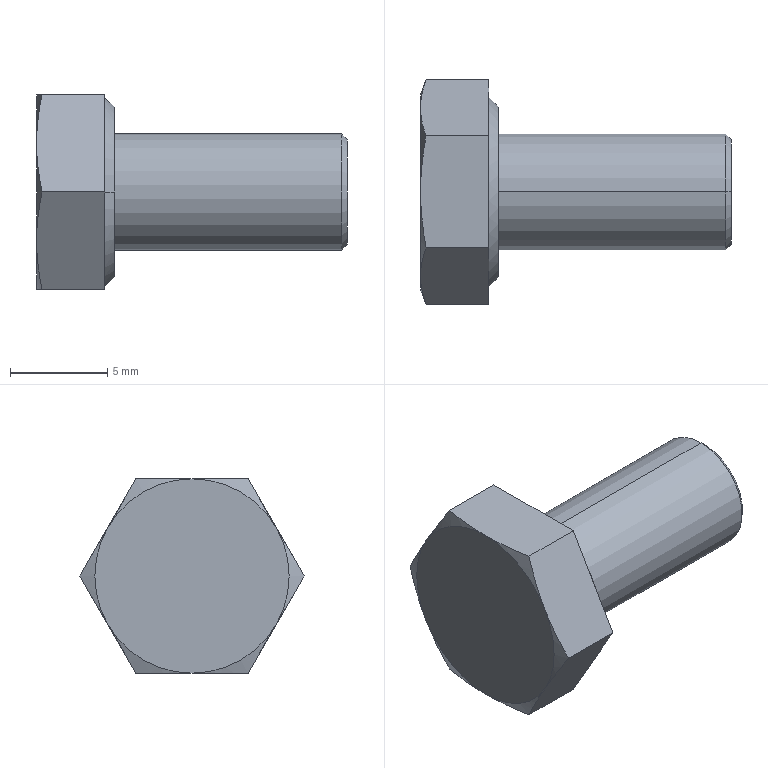Part | STEP file | hex head bolts-full thread grade c gb_GB_FASTENER_BOLT_HHBFTC M6X12-S | 1 solid | 22 faces | box 16 x 11.547 x 10 mm | volume 674.444 mm3 | cone 10 | plane 10 | cylinder 2 | commonest cylinder face diameters 6 x2
STEP:
#1=CARTESIAN_POINT('',(15.7,0.,3.));
#2=VERTEX_POINT('',#1);
#3=CARTESIAN_POINT('',(15.7,0.,-3.));
#4=VERTEX_POINT('',#3);
#5=CARTESIAN_POINT('',(15.7,0.,0.));
#6=DIRECTION('',(-1.,0.,0.));
#7=DIRECTION('',(0.,0.,1.));
#8=AXIS2_PLACEMENT_3D('',#5,#6,#7);
#9=CIRCLE('',#8,3.);
#10=EDGE_CURVE('',#2,#4,#9,.T.);
#11=ORIENTED_EDGE('',*,*,#10,.T.);
#12=CARTESIAN_POINT('',(4.,0.,-3.));
#13=VERTEX_POINT('',#12);
#14=CARTESIAN_POINT('',(16.,0.,-3.));
#15=DIRECTION('',(-1.,0.,0.));
#16=VECTOR('',#15,1000.);
#17=LINE('',#14,#16);
#18=EDGE_CURVE('',#4,#13,#17,.T.);
#19=ORIENTED_EDGE('',*,*,#18,.T.);
#20=CARTESIAN_POINT('',(4.,0.,3.));
#21=VERTEX_POINT('',#20);
#22=CARTESIAN_POINT('',(4.,0.,0.));
#23=DIRECTION('',(1.,0.,0.));
#24=DIRECTION('',(0.,0.,1.));
#25=AXIS2_PLACEMENT_3D('',#22,#23,#24);
#26=CIRCLE('',#25,3.);
#27=EDGE_CURVE('',#13,#21,#26,.T.);
#28=ORIENTED_EDGE('',*,*,#27,.T.);
#29=CARTESIAN_POINT('',(16.,0.,3.));
#30=DIRECTION('',(-1.,0.,0.));
#31=VECTOR('',#30,1000.);
#32=LINE('',#29,#31);
#33=EDGE_CURVE('',#2,#21,#32,.T.);
#34=ORIENTED_EDGE('',*,*,#33,.F.);
#35=EDGE_LOOP('',(#11,#19,#28,#34));
#36=FACE_OUTER_BOUND('',#35,.T.);
#37=CARTESIAN_POINT('',(16.,0.,0.));
#38=DIRECTION('',(-1.,0.,0.));
#39=DIRECTION('',(0.,0.,1.));
#40=AXIS2_PLACEMENT_3D('',#37,#38,#39);
#41=CYLINDRICAL_SURFACE('',#40,3.);
#42=ADVANCED_FACE('',(#36),#41,.T.);
#43=CARTESIAN_POINT('',(16.,0.,2.7));
#44=VERTEX_POINT('',#43);
#45=CARTESIAN_POINT('',(16.,0.,-2.7));
#46=VERTEX_POINT('',#45);
#47=CARTESIAN_POINT('',(16.,0.,0.));
#48=DIRECTION('',(-1.,0.,0.));
#49=DIRECTION('',(0.,0.,1.));
#50=AXIS2_PLACEMENT_3D('',#47,#48,#49);
#51=CIRCLE('',#50,2.7);
#52=EDGE_CURVE('',#44,#46,#51,.T.);
#53=ORIENTED_EDGE('',*,*,#52,.T.);
#54=CARTESIAN_POINT('',(15.7,0.,-3.));
#55=DIRECTION('',(-0.7071,0.,-0.7071));
#56=VECTOR('',#55,1000.);
#57=LINE('',#54,#56);
#58=EDGE_CURVE('',#46,#4,#57,.T.);
#59=ORIENTED_EDGE('',*,*,#58,.T.);
#60=ORIENTED_EDGE('',*,*,#10,.F.);
#61=CARTESIAN_POINT('',(15.7,0.,3.));
#62=DIRECTION('',(-0.7071,0.,0.7071));
#63=VECTOR('',#62,1000.);
#64=LINE('',#61,#63);
#65=EDGE_CURVE('',#44,#2,#64,.T.);
#66=ORIENTED_EDGE('',*,*,#65,.F.);
#67=EDGE_LOOP('',(#53,#59,#60,#66));
#68=FACE_OUTER_BOUND('',#67,.T.);
#69=CARTESIAN_POINT('',(15.7,0.,0.));
#70=DIRECTION('',(-1.,0.,0.));
#71=DIRECTION('',(0.,0.,1.));
#72=AXIS2_PLACEMENT_3D('',#69,#70,#71);
#73=CONICAL_SURFACE('',#72,3.,0.7854);
#74=ADVANCED_FACE('',(#68),#73,.T.);
#75=CARTESIAN_POINT('',(4.,4.37,0.));
#76=VERTEX_POINT('',#75);
#77=CARTESIAN_POINT('',(4.,-4.37,0.));
#78=VERTEX_POINT('',#77);
#79=CARTESIAN_POINT('',(4.,0.,0.));
#80=DIRECTION('',(1.,0.,0.));
#81=DIRECTION('',(0.,-1.,0.));
#82=AXIS2_PLACEMENT_3D('',#79,#80,#81);
#83=CIRCLE('',#82,4.37);
#84=EDGE_CURVE('',#76,#78,#83,.T.);
#85=ORIENTED_EDGE('',*,*,#84,.F.);
#86=CARTESIAN_POINT('',(3.5,4.87,0.));
#87=VERTEX_POINT('',#86);
#88=CARTESIAN_POINT('',(3.5,4.87,0.));
#89=DIRECTION('',(-0.7071,0.7071,0.));
#90=VECTOR('',#89,1000.);
#91=LINE('',#88,#90);
#92=EDGE_CURVE('',#76,#87,#91,.T.);
#93=ORIENTED_EDGE('',*,*,#92,.T.);
#94=CARTESIAN_POINT('',(3.5,-4.87,0.));
#95=VERTEX_POINT('',#94);
#96=CARTESIAN_POINT('',(3.5,0.,0.));
#97=DIRECTION('',(1.,0.,0.));
#98=DIRECTION('',(0.,-1.,0.));
#99=AXIS2_PLACEMENT_3D('',#96,#97,#98);
#100=CIRCLE('',#99,4.87);
#101=EDGE_CURVE('',#87,#95,#100,.T.);
#102=ORIENTED_EDGE('',*,*,#101,.T.);
#103=CARTESIAN_POINT('',(3.5,-4.87,0.));
#104=DIRECTION('',(-0.7071,-0.7071,0.));
#105=VECTOR('',#104,1000.);
#106=LINE('',#103,#105);
#107=EDGE_CURVE('',#78,#95,#106,.T.);
#108=ORIENTED_EDGE('',*,*,#107,.F.);
#109=EDGE_LOOP('',(#85,#93,#102,#108));
#110=FACE_OUTER_BOUND('',#109,.T.);
#111=CARTESIAN_POINT('',(3.5,0.,0.));
#112=DIRECTION('',(-1.,0.,0.));
#113=DIRECTION('',(0.,-1.,0.));
#114=AXIS2_PLACEMENT_3D('',#111,#112,#113);
#115=CONICAL_SURFACE('',#114,4.87,0.7854);
#116=ADVANCED_FACE('',(#110),#115,.T.);
#117=ORIENTED_EDGE('',*,*,#18,.F.);
#118=CARTESIAN_POINT('',(15.7,0.,0.));
#119=DIRECTION('',(-1.,0.,0.));
#120=DIRECTION('',(0.,0.,1.));
#121=AXIS2_PLACEMENT_3D('',#118,#119,#120);
#122=CIRCLE('',#121,3.);
#123=EDGE_CURVE('',#4,#2,#122,.T.);
#124=ORIENTED_EDGE('',*,*,#123,.T.);
#125=ORIENTED_EDGE('',*,*,#33,.T.);
#126=CARTESIAN_POINT('',(4.,0.,0.));
#127=DIRECTION('',(1.,0.,0.));
#128=DIRECTION('',(0.,0.,1.));
#129=AXIS2_PLACEMENT_3D('',#126,#127,#128);
#130=CIRCLE('',#129,3.);
#131=EDGE_CURVE('',#21,#13,#130,.T.);
#132=ORIENTED_EDGE('',*,*,#131,.T.);
#133=EDGE_LOOP('',(#117,#124,#125,#132));
#134=FACE_OUTER_BOUND('',#133,.T.);
#135=CARTESIAN_POINT('',(16.,0.,0.));
#136=DIRECTION('',(-1.,0.,0.));
#137=DIRECTION('',(0.,0.,1.));
#138=AXIS2_PLACEMENT_3D('',#135,#136,#137);
#139=CYLINDRICAL_SURFACE('',#138,3.);
#140=ADVANCED_FACE('',(#134),#139,.T.);
#141=ORIENTED_EDGE('',*,*,#131,.F.);
#142=ORIENTED_EDGE('',*,*,#27,.F.);
#143=EDGE_LOOP('',(#141,#142));
#144=FACE_BOUND('',#143,.T.);
#145=CARTESIAN_POINT('',(4.,0.,0.));
#146=DIRECTION('',(1.,0.,0.));
#147=DIRECTION('',(0.,-1.,0.));
#148=AXIS2_PLACEMENT_3D('',#145,#146,#147);
#149=CIRCLE('',#148,4.37);
#150=EDGE_CURVE('',#78,#76,#149,.T.);
#151=ORIENTED_EDGE('',*,*,#150,.T.);
#152=ORIENTED_EDGE('',*,*,#84,.T.);
#153=EDGE_LOOP('',(#151,#152));
#154=FACE_OUTER_BOUND('',#153,.T.);
#155=CARTESIAN_POINT('',(4.,-8.66,-5.));
#156=DIRECTION('',(1.,0.,0.));
#157=DIRECTION('',(0.,0.,-1.));
#158=AXIS2_PLACEMENT_3D('',#155,#156,#157);
#159=PLANE('',#158);
#160=ADVANCED_FACE('',(#144,#154),#159,.T.);
#161=ORIENTED_EDGE('',*,*,#58,.F.);
#162=CARTESIAN_POINT('',(16.,0.,0.));
#163=DIRECTION('',(-1.,0.,0.));
#164=DIRECTION('',(0.,0.,1.));
#165=AXIS2_PLACEMENT_3D('',#162,#163,#164);
#166=CIRCLE('',#165,2.7);
#167=EDGE_CURVE('',#46,#44,#166,.T.);
#168=ORIENTED_EDGE('',*,*,#167,.T.);
#169=ORIENTED_EDGE('',*,*,#65,.T.);
#170=ORIENTED_EDGE('',*,*,#123,.F.);
#171=EDGE_LOOP('',(#161,#168,#169,#170));
#172=FACE_OUTER_BOUND('',#171,.T.);
#173=CARTESIAN_POINT('',(15.7,0.,0.));
#174=DIRECTION('',(-1.,0.,0.));
#175=DIRECTION('',(0.,0.,1.));
#176=AXIS2_PLACEMENT_3D('',#173,#174,#175);
#177=CONICAL_SURFACE('',#176,3.,0.7854);
#178=ADVANCED_FACE('',(#172),#177,.T.);
#179=ORIENTED_EDGE('',*,*,#92,.F.);
#180=ORIENTED_EDGE('',*,*,#150,.F.);
#181=ORIENTED_EDGE('',*,*,#107,.T.);
#182=CARTESIAN_POINT('',(3.5,0.,0.));
#183=DIRECTION('',(1.,0.,0.));
#184=DIRECTION('',(0.,-1.,0.));
#185=AXIS2_PLACEMENT_3D('',#182,#183,#184);
#186=CIRCLE('',#185,4.87);
#187=EDGE_CURVE('',#95,#87,#186,.T.);
#188=ORIENTED_EDGE('',*,*,#187,.T.);
#189=EDGE_LOOP('',(#179,#180,#181,#188));
#190=FACE_OUTER_BOUND('',#189,.T.);
#191=CARTESIAN_POINT('',(3.5,0.,0.));
#192=DIRECTION('',(-1.,0.,0.));
#193=DIRECTION('',(0.,-1.,0.));
#194=AXIS2_PLACEMENT_3D('',#191,#192,#193);
#195=CONICAL_SURFACE('',#194,4.87,0.7854);
#196=ADVANCED_FACE('',(#190),#195,.T.);
#197=ORIENTED_EDGE('',*,*,#52,.F.);
#198=ORIENTED_EDGE('',*,*,#167,.F.);
#199=EDGE_LOOP('',(#197,#198));
#200=FACE_OUTER_BOUND('',#199,.T.);
#201=CARTESIAN_POINT('',(16.,0.,0.));
#202=DIRECTION('',(1.,0.,0.));
#203=DIRECTION('',(0.,0.,-1.));
#204=AXIS2_PLACEMENT_3D('',#201,#202,#203);
#205=PLANE('',#204);
#206=ADVANCED_FACE('',(#200),#205,.T.);
#207=CARTESIAN_POINT('',(3.5,5.774,0.));
#208=VERTEX_POINT('',#207);
#209=CARTESIAN_POINT('',(3.5,2.887,5.));
#210=VERTEX_POINT('',#209);
#211=CARTESIAN_POINT('',(3.5,5.774,0.));
#212=DIRECTION('',(0.,-0.5,0.866));
#213=VECTOR('',#212,1000.);
#214=LINE('',#211,#213);
#215=EDGE_CURVE('',#208,#210,#214,.T.);
#216=ORIENTED_EDGE('',*,*,#215,.T.);
#217=CARTESIAN_POINT('',(3.5,-2.887,5.));
#218=VERTEX_POINT('',#217);
#219=CARTESIAN_POINT('',(3.5,4.87,5.));
#220=DIRECTION('',(0.,-1.,0.));
#221=VECTOR('',#220,1000.);
#222=LINE('',#219,#221);
#223=EDGE_CURVE('',#210,#218,#222,.T.);
#224=ORIENTED_EDGE('',*,*,#223,.T.);
#225=CARTESIAN_POINT('',(3.5,-5.774,0.));
#226=VERTEX_POINT('',#225);
#227=CARTESIAN_POINT('',(3.5,-2.887,5.));
#228=DIRECTION('',(0.,-0.5,-0.866));
#229=VECTOR('',#228,1000.);
#230=LINE('',#227,#229);
#231=EDGE_CURVE('',#218,#226,#230,.T.);
#232=ORIENTED_EDGE('',*,*,#231,.T.);
#233=CARTESIAN_POINT('',(3.5,-2.887,-5.));
#234=VERTEX_POINT('',#233);
#235=CARTESIAN_POINT('',(3.5,-5.774,0.));
#236=DIRECTION('',(0.,0.5,-0.866));
#237=VECTOR('',#236,1000.);
#238=LINE('',#235,#237);
#239=EDGE_CURVE('',#226,#234,#238,.T.);
#240=ORIENTED_EDGE('',*,*,#239,.T.);
#241=CARTESIAN_POINT('',(3.5,2.887,-5.));
#242=VERTEX_POINT('',#241);
#243=CARTESIAN_POINT('',(3.5,4.87,-5.));
#244=DIRECTION('',(0.,1.,0.));
#245=VECTOR('',#244,1000.);
#246=LINE('',#243,#245);
#247=EDGE_CURVE('',#234,#242,#246,.T.);
#248=ORIENTED_EDGE('',*,*,#247,.T.);
#249=CARTESIAN_POINT('',(3.5,2.887,-5.));
#250=DIRECTION('',(0.,0.5,0.866));
#251=VECTOR('',#250,1000.);
#252=LINE('',#249,#251);
#253=EDGE_CURVE('',#242,#208,#252,.T.);
#254=ORIENTED_EDGE('',*,*,#253,.T.);
#255=EDGE_LOOP('',(#216,#224,#232,#240,#248,#254));
#256=FACE_OUTER_BOUND('',#255,.T.);
#257=ORIENTED_EDGE('',*,*,#187,.F.);
#258=ORIENTED_EDGE('',*,*,#101,.F.);
#259=EDGE_LOOP('',(#257,#258));
#260=FACE_BOUND('',#259,.T.);
#261=CARTESIAN_POINT('',(3.5,4.87,0.));
#262=DIRECTION('',(1.,0.,0.));
#263=DIRECTION('',(0.,0.,-1.));
#264=AXIS2_PLACEMENT_3D('',#261,#262,#263);
#265=PLANE('',#264);
#266=ADVANCED_FACE('',(#256,#260),#265,.T.);
#267=CARTESIAN_POINT('',(0.2815,-2.887,5.));
#268=VERTEX_POINT('',#267);
#269=CARTESIAN_POINT('',(4.,-2.887,5.));
#270=DIRECTION('',(-1.,0.,0.));
#271=VECTOR('',#270,1000.);
#272=LINE('',#269,#271);
#273=EDGE_CURVE('',#218,#268,#272,.T.);
#274=ORIENTED_EDGE('',*,*,#273,.F.);
#275=ORIENTED_EDGE('',*,*,#223,.F.);
#276=CARTESIAN_POINT('',(0.2815,2.887,5.));
#277=VERTEX_POINT('',#276);
#278=CARTESIAN_POINT('',(4.,2.887,5.));
#279=DIRECTION('',(1.,0.,0.));
#280=VECTOR('',#279,1000.);
#281=LINE('',#278,#280);
#282=EDGE_CURVE('',#277,#210,#281,.T.);
#283=ORIENTED_EDGE('',*,*,#282,.F.);
#284=CARTESIAN_POINT('',(0.,0.,5.));
#285=VERTEX_POINT('',#284);
#286=CARTESIAN_POINT('',(0.,0.,5.));
#287=CARTESIAN_POINT('',(0.,0.9714,5.));
#288=CARTESIAN_POINT('',(0.1078,1.932,5.));
#289=CARTESIAN_POINT('',(0.2815,2.887,5.));
#290=B_SPLINE_CURVE_WITH_KNOTS('',3,(#286,#287,#288,#289),.UNSPECIFIED.,.F.,.F.,(4,4),(0.,0.0029),.UNSPECIFIED.);
#291=EDGE_CURVE('',#285,#277,#290,.T.);
#292=ORIENTED_EDGE('',*,*,#291,.F.);
#293=CARTESIAN_POINT('',(0.2815,-2.887,5.));
#294=CARTESIAN_POINT('',(0.1078,-1.932,5.));
#295=CARTESIAN_POINT('',(0.,-0.9714,5.));
#296=CARTESIAN_POINT('',(0.,0.,5.));
#297=B_SPLINE_CURVE_WITH_KNOTS('',3,(#293,#294,#295,#296),.UNSPECIFIED.,.F.,.F.,(4,4),(0.,0.0029),.UNSPECIFIED.);
#298=EDGE_CURVE('',#268,#285,#297,.T.);
#299=ORIENTED_EDGE('',*,*,#298,.F.);
#300=EDGE_LOOP('',(#274,#275,#283,#292,#299));
#301=FACE_OUTER_BOUND('',#300,.T.);
#302=CARTESIAN_POINT('',(4.,2.887,5.));
#303=DIRECTION('',(0.,0.,-1.));
#304=DIRECTION('',(0.,1.,0.));
#305=AXIS2_PLACEMENT_3D('',#302,#303,#304);
#306=PLANE('',#305);
#307=ADVANCED_FACE('',(#301),#306,.F.);
#308=ORIENTED_EDGE('',*,*,#282,.T.);
#309=ORIENTED_EDGE('',*,*,#215,.F.);
#310=CARTESIAN_POINT('',(0.2815,5.774,0.));
#311=VERTEX_POINT('',#310);
#312=CARTESIAN_POINT('',(4.,5.774,0.));
#313=DIRECTION('',(1.,0.,0.));
#314=VECTOR('',#313,1000.);
#315=LINE('',#312,#314);
#316=EDGE_CURVE('',#311,#208,#315,.T.);
#317=ORIENTED_EDGE('',*,*,#316,.F.);
#318=CARTESIAN_POINT('',(0.,4.33,2.5));
#319=VERTEX_POINT('',#318);
#320=CARTESIAN_POINT('',(0.,4.33,2.5));
#321=CARTESIAN_POINT('',(0.,4.816,1.659));
#322=CARTESIAN_POINT('',(0.1078,5.296,0.8266));
#323=CARTESIAN_POINT('',(0.2815,5.774,0.));
#324=B_SPLINE_CURVE_WITH_KNOTS('',3,(#320,#321,#322,#323),.UNSPECIFIED.,.F.,.F.,(4,4),(0.,0.0029),.UNSPECIFIED.);
#325=EDGE_CURVE('',#319,#311,#324,.T.);
#326=ORIENTED_EDGE('',*,*,#325,.F.);
#327=CARTESIAN_POINT('',(0.2815,2.887,5.));
#328=CARTESIAN_POINT('',(0.1078,3.364,4.173));
#329=CARTESIAN_POINT('',(0.,3.844,3.341));
#330=CARTESIAN_POINT('',(0.,4.33,2.5));
#331=B_SPLINE_CURVE_WITH_KNOTS('',3,(#327,#328,#329,#330),.UNSPECIFIED.,.F.,.F.,(4,4),(0.,0.0029),.UNSPECIFIED.);
#332=EDGE_CURVE('',#277,#319,#331,.T.);
#333=ORIENTED_EDGE('',*,*,#332,.F.);
#334=EDGE_LOOP('',(#308,#309,#317,#326,#333));
#335=FACE_OUTER_BOUND('',#334,.T.);
#336=CARTESIAN_POINT('',(4.,5.774,0.));
#337=DIRECTION('',(0.,-0.866,-0.5));
#338=DIRECTION('',(0.,0.5,-0.866));
#339=AXIS2_PLACEMENT_3D('',#336,#337,#338);
#340=PLANE('',#339);
#341=ADVANCED_FACE('',(#335),#340,.F.);
#342=ORIENTED_EDGE('',*,*,#316,.T.);
#343=ORIENTED_EDGE('',*,*,#253,.F.);
#344=CARTESIAN_POINT('',(0.2815,2.887,-5.));
#345=VERTEX_POINT('',#344);
#346=CARTESIAN_POINT('',(4.,2.887,-5.));
#347=DIRECTION('',(1.,0.,0.));
#348=VECTOR('',#347,1000.);
#349=LINE('',#346,#348);
#350=EDGE_CURVE('',#345,#242,#349,.T.);
#351=ORIENTED_EDGE('',*,*,#350,.F.);
#352=CARTESIAN_POINT('',(0.,4.33,-2.5));
#353=VERTEX_POINT('',#352);
#354=CARTESIAN_POINT('',(0.,4.33,-2.5));
#355=CARTESIAN_POINT('',(0.,3.844,-3.341));
#356=CARTESIAN_POINT('',(0.1078,3.364,-4.173));
#357=CARTESIAN_POINT('',(0.2815,2.887,-5.));
#358=B_SPLINE_CURVE_WITH_KNOTS('',3,(#354,#355,#356,#357),.UNSPECIFIED.,.F.,.F.,(4,4),(0.,0.0029),.UNSPECIFIED.);
#359=EDGE_CURVE('',#353,#345,#358,.T.);
#360=ORIENTED_EDGE('',*,*,#359,.F.);
#361=CARTESIAN_POINT('',(0.2815,5.774,0.));
#362=CARTESIAN_POINT('',(0.1078,5.296,-0.8266));
#363=CARTESIAN_POINT('',(0.,4.816,-1.659));
#364=CARTESIAN_POINT('',(0.,4.33,-2.5));
#365=B_SPLINE_CURVE_WITH_KNOTS('',3,(#361,#362,#363,#364),.UNSPECIFIED.,.F.,.F.,(4,4),(0.,0.0029),.UNSPECIFIED.);
#366=EDGE_CURVE('',#311,#353,#365,.T.);
#367=ORIENTED_EDGE('',*,*,#366,.F.);
#368=EDGE_LOOP('',(#342,#343,#351,#360,#367));
#369=FACE_OUTER_BOUND('',#368,.T.);
#370=CARTESIAN_POINT('',(4.,2.887,-5.));
#371=DIRECTION('',(0.,-0.866,0.5));
#372=DIRECTION('',(0.,-0.5,-0.866));
#373=AXIS2_PLACEMENT_3D('',#370,#371,#372);
#374=PLANE('',#373);
#375=ADVANCED_FACE('',(#369),#374,.F.);
#376=ORIENTED_EDGE('',*,*,#350,.T.);
#377=ORIENTED_EDGE('',*,*,#247,.F.);
#378=CARTESIAN_POINT('',(0.2815,-2.887,-5.));
#379=VERTEX_POINT('',#378);
#380=CARTESIAN_POINT('',(4.,-2.887,-5.));
#381=DIRECTION('',(1.,0.,0.));
#382=VECTOR('',#381,1000.);
#383=LINE('',#380,#382);
#384=EDGE_CURVE('',#379,#234,#383,.T.);
#385=ORIENTED_EDGE('',*,*,#384,.F.);
#386=CARTESIAN_POINT('',(0.,0.,-5.));
#387=VERTEX_POINT('',#386);
#388=CARTESIAN_POINT('',(0.,0.,-5.));
#389=CARTESIAN_POINT('',(0.,-0.9714,-5.));
#390=CARTESIAN_POINT('',(0.1078,-1.932,-5.));
#391=CARTESIAN_POINT('',(0.2815,-2.887,-5.));
#392=B_SPLINE_CURVE_WITH_KNOTS('',3,(#388,#389,#390,#391),.UNSPECIFIED.,.F.,.F.,(4,4),(0.,0.0029),.UNSPECIFIED.);
#393=EDGE_CURVE('',#387,#379,#392,.T.);
#394=ORIENTED_EDGE('',*,*,#393,.F.);
#395=CARTESIAN_POINT('',(0.2815,2.887,-5.));
#396=CARTESIAN_POINT('',(0.1078,1.932,-5.));
#397=CARTESIAN_POINT('',(0.,0.9714,-5.));
#398=CARTESIAN_POINT('',(0.,0.,-5.));
#399=B_SPLINE_CURVE_WITH_KNOTS('',3,(#395,#396,#397,#398),.UNSPECIFIED.,.F.,.F.,(4,4),(0.,0.0029),.UNSPECIFIED.);
#400=EDGE_CURVE('',#345,#387,#399,.T.);
#401=ORIENTED_EDGE('',*,*,#400,.F.);
#402=EDGE_LOOP('',(#376,#377,#385,#394,#401));
#403=FACE_OUTER_BOUND('',#402,.T.);
#404=CARTESIAN_POINT('',(4.,-2.887,-5.));
#405=DIRECTION('',(0.,0.,1.));
#406=DIRECTION('',(1.,0.,0.));
#407=AXIS2_PLACEMENT_3D('',#404,#405,#406);
#408=PLANE('',#407);
#409=ADVANCED_FACE('',(#403),#408,.F.);
#410=ORIENTED_EDGE('',*,*,#384,.T.);
#411=ORIENTED_EDGE('',*,*,#239,.F.);
#412=CARTESIAN_POINT('',(0.2815,-5.774,0.));
#413=VERTEX_POINT('',#412);
#414=CARTESIAN_POINT('',(4.,-5.774,0.));
#415=DIRECTION('',(1.,0.,0.));
#416=VECTOR('',#415,1000.);
#417=LINE('',#414,#416);
#418=EDGE_CURVE('',#413,#226,#417,.T.);
#419=ORIENTED_EDGE('',*,*,#418,.F.);
#420=CARTESIAN_POINT('',(0.,-4.33,-2.5));
#421=VERTEX_POINT('',#420);
#422=CARTESIAN_POINT('',(0.,-4.33,-2.5));
#423=CARTESIAN_POINT('',(0.,-4.816,-1.659));
#424=CARTESIAN_POINT('',(0.1078,-5.296,-0.8266));
#425=CARTESIAN_POINT('',(0.2815,-5.774,0.));
#426=B_SPLINE_CURVE_WITH_KNOTS('',3,(#422,#423,#424,#425),.UNSPECIFIED.,.F.,.F.,(4,4),(0.,0.0029),.UNSPECIFIED.);
#427=EDGE_CURVE('',#421,#413,#426,.T.);
#428=ORIENTED_EDGE('',*,*,#427,.F.);
#429=CARTESIAN_POINT('',(0.2815,-2.887,-5.));
#430=CARTESIAN_POINT('',(0.1078,-3.364,-4.173));
#431=CARTESIAN_POINT('',(0.,-3.844,-3.341));
#432=CARTESIAN_POINT('',(0.,-4.33,-2.5));
#433=B_SPLINE_CURVE_WITH_KNOTS('',3,(#429,#430,#431,#432),.UNSPECIFIED.,.F.,.F.,(4,4),(0.,0.0029),.UNSPECIFIED.);
#434=EDGE_CURVE('',#379,#421,#433,.T.);
#435=ORIENTED_EDGE('',*,*,#434,.F.);
#436=EDGE_LOOP('',(#410,#411,#419,#428,#435));
#437=FACE_OUTER_BOUND('',#436,.T.);
#438=CARTESIAN_POINT('',(4.,-5.774,0.));
#439=DIRECTION('',(0.,0.866,0.5));
#440=DIRECTION('',(0.,-0.5,0.866));
#441=AXIS2_PLACEMENT_3D('',#438,#439,#440);
#442=PLANE('',#441);
#443=ADVANCED_FACE('',(#437),#442,.F.);
#444=ORIENTED_EDGE('',*,*,#418,.T.);
#445=ORIENTED_EDGE('',*,*,#231,.F.);
#446=ORIENTED_EDGE('',*,*,#273,.T.);
#447=CARTESIAN_POINT('',(0.,-4.33,2.5));
#448=VERTEX_POINT('',#447);
#449=CARTESIAN_POINT('',(0.,-4.33,2.5));
#450=CARTESIAN_POINT('',(0.,-3.844,3.341));
#451=CARTESIAN_POINT('',(0.1078,-3.364,4.173));
#452=CARTESIAN_POINT('',(0.2815,-2.887,5.));
#453=B_SPLINE_CURVE_WITH_KNOTS('',3,(#449,#450,#451,#452),.UNSPECIFIED.,.F.,.F.,(4,4),(0.,0.0029),.UNSPECIFIED.);
#454=EDGE_CURVE('',#448,#268,#453,.T.);
#455=ORIENTED_EDGE('',*,*,#454,.F.);
#456=CARTESIAN_POINT('',(0.2815,-5.774,0.));
#457=CARTESIAN_POINT('',(0.1078,-5.296,0.8266));
#458=CARTESIAN_POINT('',(0.,-4.816,1.659));
#459=CARTESIAN_POINT('',(0.,-4.33,2.5));
#460=B_SPLINE_CURVE_WITH_KNOTS('',3,(#456,#457,#458,#459),.UNSPECIFIED.,.F.,.F.,(4,4),(0.,0.0029),.UNSPECIFIED.);
#461=EDGE_CURVE('',#413,#448,#460,.T.);
#462=ORIENTED_EDGE('',*,*,#461,.F.);
#463=EDGE_LOOP('',(#444,#445,#446,#455,#462));
#464=FACE_OUTER_BOUND('',#463,.T.);
#465=CARTESIAN_POINT('',(4.,-2.887,5.));
#466=DIRECTION('',(0.,0.866,-0.5));
#467=DIRECTION('',(0.,0.5,0.866));
#468=AXIS2_PLACEMENT_3D('',#465,#466,#467);
#469=PLANE('',#468);
#470=ADVANCED_FACE('',(#464),#469,.F.);
#471=ORIENTED_EDGE('',*,*,#298,.T.);
#472=CARTESIAN_POINT('',(0.,0.,0.));
#473=DIRECTION('',(1.,0.,0.));
#474=DIRECTION('',(0.,0.,-1.));
#475=AXIS2_PLACEMENT_3D('',#472,#473,#474);
#476=CIRCLE('',#475,5.);
#477=EDGE_CURVE('',#285,#448,#476,.T.);
#478=ORIENTED_EDGE('',*,*,#477,.T.);
#479=ORIENTED_EDGE('',*,*,#454,.T.);
#480=EDGE_LOOP('',(#471,#478,#479));
#481=FACE_OUTER_BOUND('',#480,.T.);
#482=CARTESIAN_POINT('',(0.2832,0.,0.));
#483=DIRECTION('',(1.,0.,0.));
#484=DIRECTION('',(0.,0.,-1.));
#485=AXIS2_PLACEMENT_3D('',#482,#483,#484);
#486=CONICAL_SURFACE('',#485,5.778,1.222);
#487=ADVANCED_FACE('',(#481),#486,.T.);
#488=CARTESIAN_POINT('',(0.,0.,0.));
#489=DIRECTION('',(1.,0.,0.));
#490=DIRECTION('',(0.,0.,-1.));
#491=AXIS2_PLACEMENT_3D('',#488,#489,#490);
#492=CIRCLE('',#491,5.);
#493=EDGE_CURVE('',#319,#285,#492,.T.);
#494=ORIENTED_EDGE('',*,*,#493,.T.);
#495=ORIENTED_EDGE('',*,*,#291,.T.);
#496=ORIENTED_EDGE('',*,*,#332,.T.);
#497=EDGE_LOOP('',(#494,#495,#496));
#498=FACE_OUTER_BOUND('',#497,.T.);
#499=CARTESIAN_POINT('',(0.2832,0.,0.));
#500=DIRECTION('',(1.,0.,0.));
#501=DIRECTION('',(0.,0.,-1.));
#502=AXIS2_PLACEMENT_3D('',#499,#500,#501);
#503=CONICAL_SURFACE('',#502,5.778,1.222);
#504=ADVANCED_FACE('',(#498),#503,.T.);
#505=CARTESIAN_POINT('',(0.,0.,0.));
#506=DIRECTION('',(1.,0.,0.));
#507=DIRECTION('',(0.,0.,-1.));
#508=AXIS2_PLACEMENT_3D('',#505,#506,#507);
#509=CIRCLE('',#508,5.);
#510=EDGE_CURVE('',#353,#319,#509,.T.);
#511=ORIENTED_EDGE('',*,*,#510,.T.);
#512=ORIENTED_EDGE('',*,*,#325,.T.);
#513=ORIENTED_EDGE('',*,*,#366,.T.);
#514=EDGE_LOOP('',(#511,#512,#513));
#515=FACE_OUTER_BOUND('',#514,.T.);
#516=CARTESIAN_POINT('',(0.2832,0.,0.));
#517=DIRECTION('',(1.,0.,0.));
#518=DIRECTION('',(0.,0.,-1.));
#519=AXIS2_PLACEMENT_3D('',#516,#517,#518);
#520=CONICAL_SURFACE('',#519,5.778,1.222);
#521=ADVANCED_FACE('',(#515),#520,.T.);
#522=CARTESIAN_POINT('',(0.,0.,0.));
#523=DIRECTION('',(1.,0.,0.));
#524=DIRECTION('',(0.,0.,-1.));
#525=AXIS2_PLACEMENT_3D('',#522,#523,#524);
#526=CIRCLE('',#525,5.);
#527=EDGE_CURVE('',#387,#353,#526,.T.);
#528=ORIENTED_EDGE('',*,*,#527,.T.);
#529=ORIENTED_EDGE('',*,*,#359,.T.);
#530=ORIENTED_EDGE('',*,*,#400,.T.);
#531=EDGE_LOOP('',(#528,#529,#530));
#532=FACE_OUTER_BOUND('',#531,.T.);
#533=CARTESIAN_POINT('',(0.2832,0.,0.));
#534=DIRECTION('',(1.,0.,0.));
#535=DIRECTION('',(0.,0.,-1.));
#536=AXIS2_PLACEMENT_3D('',#533,#534,#535);
#537=CONICAL_SURFACE('',#536,5.778,1.222);
#538=ADVANCED_FACE('',(#532),#537,.T.);
#539=ORIENTED_EDGE('',*,*,#434,.T.);
#540=CARTESIAN_POINT('',(0.,0.,0.));
#541=DIRECTION('',(1.,0.,0.));
#542=DIRECTION('',(0.,0.,-1.));
#543=AXIS2_PLACEMENT_3D('',#540,#541,#542);
#544=CIRCLE('',#543,5.);
#545=EDGE_CURVE('',#421,#387,#544,.T.);
#546=ORIENTED_EDGE('',*,*,#545,.T.);
#547=ORIENTED_EDGE('',*,*,#393,.T.);
#548=EDGE_LOOP('',(#539,#546,#547));
#549=FACE_OUTER_BOUND('',#548,.T.);
#550=CARTESIAN_POINT('',(0.2832,0.,0.));
#551=DIRECTION('',(1.,0.,0.));
#552=DIRECTION('',(0.,0.,-1.));
#553=AXIS2_PLACEMENT_3D('',#550,#551,#552);
#554=CONICAL_SURFACE('',#553,5.778,1.222);
#555=ADVANCED_FACE('',(#549),#554,.T.);
#556=ORIENTED_EDGE('',*,*,#461,.T.);
#557=CARTESIAN_POINT('',(0.,0.,0.));
#558=DIRECTION('',(1.,0.,0.));
#559=DIRECTION('',(0.,0.,-1.));
#560=AXIS2_PLACEMENT_3D('',#557,#558,#559);
#561=CIRCLE('',#560,5.);
#562=EDGE_CURVE('',#448,#421,#561,.T.);
#563=ORIENTED_EDGE('',*,*,#562,.T.);
#564=ORIENTED_EDGE('',*,*,#427,.T.);
#565=EDGE_LOOP('',(#556,#563,#564));
#566=FACE_OUTER_BOUND('',#565,.T.);
#567=CARTESIAN_POINT('',(0.2832,0.,0.));
#568=DIRECTION('',(1.,0.,0.));
#569=DIRECTION('',(0.,0.,-1.));
#570=AXIS2_PLACEMENT_3D('',#567,#568,#569);
#571=CONICAL_SURFACE('',#570,5.778,1.222);
#572=ADVANCED_FACE('',(#566),#571,.T.);
#573=ORIENTED_EDGE('',*,*,#545,.F.);
#574=ORIENTED_EDGE('',*,*,#562,.F.);
#575=ORIENTED_EDGE('',*,*,#477,.F.);
#576=ORIENTED_EDGE('',*,*,#493,.F.);
#577=ORIENTED_EDGE('',*,*,#510,.F.);
#578=ORIENTED_EDGE('',*,*,#527,.F.);
#579=EDGE_LOOP('',(#573,#574,#575,#576,#577,#578));
#580=FACE_OUTER_BOUND('',#579,.T.);
#581=CARTESIAN_POINT('',(0.,-8.66,-5.));
#582=DIRECTION('',(1.,0.,0.));
#583=DIRECTION('',(0.,0.,-1.));
#584=AXIS2_PLACEMENT_3D('',#581,#582,#583);
#585=PLANE('',#584);
#586=ADVANCED_FACE('',(#580),#585,.F.);
#587=CLOSED_SHELL('',(#42,#74,#116,#140,#160,#178,#196,#206,#266,#307,#341,#375,#409,#443,#470,#487,#504,#521,#538,#555,#572,#586));
#588=MANIFOLD_SOLID_BREP('',#587);
#589=CARTESIAN_POINT('',(0.,0.,0.));
#590=DIRECTION('',(0.,0.,1.));
#591=DIRECTION('',(1.,0.,0.));
#592=AXIS2_PLACEMENT_3D('',#589,#590,#591);
#593=(LENGTH_UNIT()NAMED_UNIT(*)SI_UNIT(.MILLI.,.METRE.));
#594=UNCERTAINTY_MEASURE_WITH_UNIT(LENGTH_MEASURE(0.00001),#593,'','');
#595=(NAMED_UNIT(*)PLANE_ANGLE_UNIT()SI_UNIT($,.RADIAN.));
#596=(NAMED_UNIT(*)SI_UNIT($,.STERADIAN.)SOLID_ANGLE_UNIT());
#597=(GEOMETRIC_REPRESENTATION_CONTEXT(3)GLOBAL_UNCERTAINTY_ASSIGNED_CONTEXT((#594))GLOBAL_UNIT_ASSIGNED_CONTEXT((#593,#595,#596))REPRESENTATION_CONTEXT('',''));
#598=ADVANCED_BREP_SHAPE_REPRESENTATION('',(#588,#592),#597);